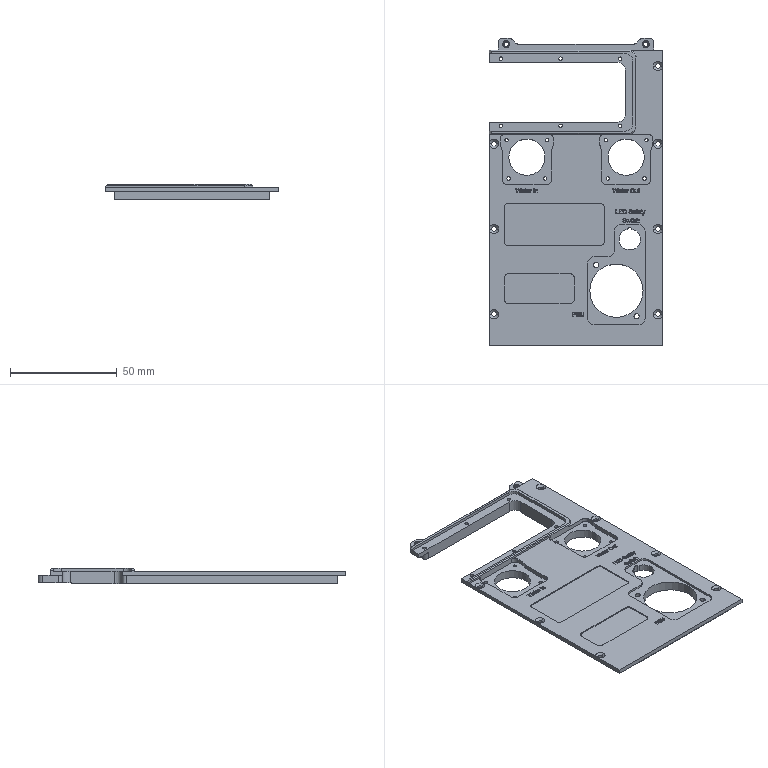NC program | NX | posted with a generic post | part box 81.5 x 144.28 x 7.5 mm
Lines 91 to 933 of 9048:
(ADAPTIVE_MILLING , TOOL : D6开粗)
N156 T01 M6
N158 G54
N160 G17 G0 G90 X-68.746 Y48.054 S6500 M3
N162 G43 Z50. H1
N164 Z-6.
N166 G94 G1 X-68.744 Y48.004 Z-6.312 F2500.
N168 X-68.741 Y47.954 Z-6.436
N170 X-68.739 Y47.904 Z-6.527
N172 X-68.736 Y47.854 Z-6.6
N174 X-68.734 Y47.804 Z-6.661
N176 X-68.731 Y47.754 Z-6.714
N178 X-68.729 Y47.704 Z-6.76
N180 X-68.727 Y47.654 Z-6.8
N182 X-68.724 Y47.604 Z-6.835
N184 X-68.722 Y47.554 Z-6.866
N186 X-68.719 Y47.504 Z-6.893
N188 X-68.717 Y47.454 Z-6.917
N190 X-68.714 Y47.404 Z-6.937
N192 X-68.712 Y47.354 Z-6.954
N194 X-68.709 Y47.305 Z-6.968
N196 X-68.707 Y47.255 Z-6.98
N198 X-68.704 Y47.205 Z-6.989
N200 X-68.702 Y47.155 Z-6.995
N202 X-68.699 Y47.105 Z-6.999
N204 X-68.697 Y47.055 Z-7.
N206 X-68.648 Y46.067
N208 G3 X-68.292 Y45.545 R0.607
N210 X-66.048 Y45.051 R6.544
N212 X-59.226 Y44.903 R95.551
N214 G1 X-55.089 Y44.901
N216 X72.351 Y44.899
N218 G2 X74.896 Y43.394 R3.392
N220 X76.098 Y40.132 R7.391
N222 X76.382 Y35.059 R37.58
N224 G1 X76.399 Y28.399
N226 X76.398 Y-40.835
N228 G2 X74.941 Y-43.359 R3.368
N230 X71.646 Y-44.596 R7.3
N232 X66.483 Y-44.883 R37.738
N234 G1 X59.103 Y-44.9
N236 X-72.29 Y-44.899
N238 G2 X-74.864 Y-43.448 R3.358
N240 X-76.09 Y-40.197 R7.25
N242 X-76.381 Y-35.079 R37.036
N244 G1 X-76.399 Y-28.149
N246 X-76.398 Y40.791
N248 G2 X-74.982 Y43.337 R3.339
N250 X-71.651 Y44.599 R7.234
N252 X-68.063 Y44.633 R12.649
N254 G3 X-59.713 Y44.31 R86.176
N256 G1 X-53.424 Y44.301
N258 X70.551 Y44.299
N260 G2 X74.189 Y42.173 R4.492
N262 X75.473 Y38.461 R9.024
N264 X75.775 Y33.209 R40.848
N266 G1 X75.799 Y25.53
N268 X75.797 Y-39.05
N270 G2 X73.654 Y-42.701 R4.49
N272 X69.98 Y-43.971 R9.023
N274 X64.233 Y-44.281 R43.718
N276 G1 X56.882 Y-44.3
N278 X-70.56 Y-44.298
N280 G2 X-72.366 Y-43.87 R5.009
N282 G1 X-72.955 Y-43.793
N284 X-73.715 Y-43.478
N286 X-74.367 Y-42.977
N288 X-74.868 Y-42.325
N290 G2 X-75.378 Y-40.504 R5.143
N292 X-75.772 Y-34.221 R45.821
N294 G1 X-75.799 Y-26.391
N296 X-75.798 Y39.061
N298 G2 X-75.25 Y41.083 R4.874
N300 G1 X-75.183 Y41.565
N302 X-74.868 Y42.325
N304 X-74.367 Y42.977
N306 X-73.715 Y43.478
N308 X-72.955 Y43.793
N310 G2 X-67.603 Y43.95 R23.279
N312 G1 X-66.688 Y43.9
N314 X66.591
N316 G3 X69.451 Y43.718 R34.087
N318 G2 X73.692 Y40.889 R5.336
N320 X74.91 Y36.767 R11.057
N322 G3 X75.195 Y35.482 R4.36
N324 G1 X75.29 Y34.499
N326 G2 X75.216 Y28.517 R176.845
N328 G1 X75.2 Y23.589
N330 X75.201 Y-30.365
N332 X75.29 Y-31.329
N334 G2 X75.184 Y-38.04 R148.514
N336 X72.364 Y-42.201 R5.303
N338 X68.371 Y-43.397 R10.985
N340 G1 X67.405 Y-43.793
N342 X66.589 Y-43.9
N344 X60.839
N346 G3 X57.254 Y-43.723 R30.565
N348 G1 X51.794 Y-43.7
N350 X33.975 Y-43.701
N352 G2 X32.839 Y-43.9 R6.236
N354 G1 X-72.141
N356 X-72.955 Y-43.793
N358 X-73.715 Y-43.478
N360 X-74.367 Y-42.977
N362 X-74.868 Y-42.325
N364 X-75.183 Y-41.565
N366 X-75.29 Y-40.749
N368 Y40.751
N370 X-75.183 Y41.565
N372 X-74.868 Y42.325
N374 X-74.367 Y42.977
N376 X-73.715 Y43.478
N378 X-72.955 Y43.793
N380 X-72.14 Y43.9
N382 X-66.65
N384 G3 X-66.063 Y44.357 R0.607
N386 G1 X-65.981 Y44.693
N388 X-65.882 Y45.024
N390 G2 X-65.333 Y45.373 R0.607
N392 G1 X-65.283 Z-6.999
N394 X-65.233 Z-6.995
N396 X-65.183 Z-6.989
N398 X-65.133 Z-6.98
N400 X-65.083 Z-6.968
N402 X-65.033 Z-6.954
N404 X-64.983 Z-6.937
N406 X-64.933 Z-6.917
N408 X-64.883 Z-6.893
N410 X-64.833 Z-6.866
N412 X-64.783 Z-6.835
N414 X-64.733 Z-6.8
N416 X-64.683 Z-6.76
N418 X-64.633 Z-6.714
N420 X-64.583 Z-6.661
N422 X-64.533 Z-6.6
N424 X-64.483 Z-6.527
N426 X-64.433 Z-6.436
N428 X-64.383 Z-6.312
N430 X-64.333 Z-6.
N432 G0 Z50.
N434 X64.727
N436 Z-6.
N438 G1 X64.777 Z-6.312
N440 X64.827 Z-6.436
N442 X64.877 Z-6.527
N444 X64.927 Z-6.6
N446 X64.977 Z-6.661
N448 X65.027 Z-6.714
N450 X65.077 Z-6.76
N452 X65.127 Z-6.8
N454 X65.177 Z-6.835
N456 X65.227 Z-6.866
N458 X65.277 Z-6.893
N460 X65.327 Z-6.917
N462 X65.377 Z-6.937
N464 X65.427 Z-6.954
N466 X65.477 Z-6.968
N468 X65.527 Z-6.98
N470 X65.577 Z-6.989
N472 X65.627 Z-6.995
N474 X65.677 Z-6.999
N476 X65.727 Z-7.
N478 G2 X66.301 Y44.962 R0.607
N480 G1 X66.542 Y44.248
N482 G3 X67.037 Y43.841 R0.607
N484 G2 X67.915 Y43.589 R2.444
N486 X70.276 Y42.804 R12.832
N488 X73.485 Y39.109 R6.8
N490 G3 X73.88 Y38.033 R13.5
N492 G2 X74.915 Y36.429 R5.884
N494 G1 X74.979 Y36.213
N496 X74.915 Y36.429
N498 G3 X73.814 Y38.112 R6.02
N500 X72.573 Y40.063 R173.318
N502 X69.102 Y42.699 R7.546
N504 G2 X68.817 Y42.977 R1.185
N506 G1 X68.165 Y43.478
N508 X67.791 Y43.633
N510 X68.165 Y43.478
N512 X68.817 Y42.977
N514 G3 X70.003 Y41.788 R6.694
N516 G2 X72.3 Y39.19 R15.9
N518 G3 X73.093 Y38.719 R15.073
N520 G1 X73.844 Y38.078
N522 G3 X72.277 Y39.181 R5.882
N524 G2 X70.58 Y40.741 R21.995
N526 X69.589 Y41.694 R16.506
N528 G1 X69.318 Y42.325
N530 X69.044 Y42.682
N532 G2 X69.555 Y41.754 R2.503
N534 G3 X71.156 Y39.578 R6.152
N536 G1 X72.311 Y39.161
N538 G3 X71.077 Y39.591 R36.922
N540 G2 X69.708 Y41.029 R3.409
N542 G1 X69.633 Y41.565
N544 G3 X69.859 Y40.484 R3.332
N546 X70.584 Y39.633 R1.822
N548 X71.293 Y39.519 R8.72
N550 G2 X70.47 Y39.659 R3.567
N552 X69.74 Y40.571 R1.303
N554 G1 X69.722 Y40.883
N556 G3 X69.767 Y40.25 R10.794
N558 X70.636 Y39.605 R0.853
N560 G2 X69.832 Y39.978 R0.96
N562 X69.74 Y40.416 R1.044
N564 G3 X69.832 Y39.978 R0.826
N566 X70.369 Y39.64 R0.728
N568 G2 X72.233 Y39.205 R5.896
N570 X73.844 Y38.078 R5.987
N572 X74.915 Y36.429 R5.987
N574 X75.29 Y34.499 R5.992
N576 G1 X75.286 Y31.283
N578 G2 X74.958 Y29.535 R5.673
N580 G3 X74.639 Y25.742 R21.469
N582 X74.6 Y18.775 R599.147
N584 G1 X74.601 Y-28.654
N586 G3 X74.992 Y-29.601 R4.451
N588 G1 X75.209 Y-30.428
N590 G3 X74.605 Y-28.761 R5.835
N592 G2 X74.307 Y-26.632 R7.842
N594 X74.239 Y-20.148 R199.676
N596 G1 X74.242 Y21.156
N598 G2 X74.404 Y27.864 R85.907
N600 X74.528 Y28.666 R3.801
N602 G3 X74.989 Y29.658 R3.993
N604 G2 X74.528 Y28.666 R3.993
N606 G3 X73.882 Y26.464 R5.45
N608 X73.65 Y20.651 R53.719
N610 G1 X73.64 Y14.365
N612 X73.642 Y-21.63
N614 G3 X73.791 Y-27.159 R61.12
N616 X73.988 Y-27.912 R1.5
N618 G2 X74.627 Y-28.801 R8.268
N620 G3 X73.898 Y-27.81 R6.471
N622 G2 X73.447 Y-25.976 R4.929
N624 X73.283 Y-20.232 R65.741
N626 G1 X73.28 Y-15.738
N628 X73.282 Y17.558
N630 G2 X73.432 Y25.243 R116.247
N632 X73.887 Y27.799 R9.722
N634 G1 X74.421 Y28.466
N636 G3 X73.542 Y27.303 R7.221
N638 X72.896 Y24.509 R8.56
N640 X72.688 Y17.82 R77.087
N642 G1 X72.68 Y11.89
N644 X72.682 Y-18.841
N646 G3 X72.825 Y-25.216 R86.495
N648 X73.151 Y-27.015 R7.72
N650 X73.934 Y-27.852 R7.987
N652 G2 X73.078 Y-26.946 R10.433
N654 X72.526 Y-24.825 R5.793
N656 G1 X72.49 Y-24.491
N658 X72.492 Y23.081
N660 G2 X73.042 Y26.737 R12.308
N662 X73.243 Y27.148 R2.48
N664 G1 X73.781 Y27.686
N666 G3 X72.831 Y26.652 R6.454
N668 X72.49 Y25.84 R2.8
N670 G1 Y22.96
N672 X72.504 Y26.094
N674 G2 X72.707 Y26.612 R1.124
N676 G1 X73.057 Y26.962
N678 G3 X72.547 Y26.372 R2.142
N680 X72.49 Y25.951 R1.722
N682 X72.79 Y25.431 R0.602
N684 G1 X72.971 Y25.326
N686 X73.443 Y25.058 Z-6.954
N688 X73.908 Y24.777 Z-6.908
N690 X73.975 Y24.713 Z-6.9
N692 G2 X74.131 Y24.31 R0.607 F15000.
N694 G1 Y-22.85
N696 G2 X73.974 Y-23.255 R0.607
N698 G1 X73.81 Y-23.383 Z-6.918 F2500.
N700 X73.63 Y-23.487 Z-6.935
N702 X72.971 Y-23.87 Z-7.
N704 X72.704 Y-24.037
N706 G3 X72.49 Y-24.491 R0.604
N708 X72.535 Y-26.276 R11.945
N710 X72.709 Y-26.614 R0.96
N712 G1 X73.186 Y-27.091
N714 G2 X72.547 Y-26.372 R3.179
N716 X72.49 Y-25.908 R1.641
N718 G3 X72.547 Y-26.372 R1.116
N720 G1 X72.709 Y-26.614
N722 G2 X74.13 Y-28.072 R49.423
N724 X75.29 Y-31.329 R5.356
N726 G1 X75.286 Y-34.546
N728 G2 X74.957 Y-36.303 R5.7
N730 X74.157 Y-38.937 R9.519
N732 X70.548 Y-41.997 R6.736
N734 G3 X69.239 Y-42.484 R25.069
N736 X68.817 Y-42.977 R2.517
N738 G1 X68.165 Y-43.478
N740 X67.999 Y-43.547
N742 X68.165 Y-43.478
N744 X68.817 Y-42.977
N746 G2 X69.794 Y-42.093 R2.317
N748 G3 X72.4 Y-40.32 R11.44
N750 X73.969 Y-37.92 R7.475
N752 X74.978 Y-36.216 R4.84
N754 G2 X73.491 Y-38.392 R4.973
N756 X70.015 Y-41.2 R19.409
N758 G3 X69.628 Y-41.576 R1.142
N760 G1 X69.318 Y-42.325
N762 X69.154 Y-42.539
N764 X69.318 Y-42.325
N766 G2 X69.732 Y-41.375 R6.637
N768 X71.329 Y-39.882 R11.928
N770 X72.09 Y-39.253 R4.923
N772 G3 X73.604 Y-38.283 R4.85
N774 G2 X71.633 Y-39.411 R4.853
N776 G3 X69.798 Y-40.736 R5.104
N778 X69.633 Y-41.565 R2.455
N780 G2 X69.782 Y-40.696 R3.509
N782 X70.945 Y-39.574 R2.827
N784 G3 X71.72 Y-39.377 R3.103
N786 G2 X70.739 Y-39.602 R3.849
N788 G3 X69.778 Y-40.339 R1.497
N790 X69.722 Y-40.885 R4.559
N792 G1 X69.744 Y-40.38
N794 G2 X70.467 Y-39.627 R1.11
N796 G1 X70.868 Y-39.575
N798 G3 X70.028 Y-39.769 R2.032
N800 X69.74 Y-40.506 R0.77
N802 G1 X69.742 Y-40.316
N804 X69.771 Y-40.128
N806 G2 X70.095 Y-39.729 R0.647
N808 X70.813 Y-39.907 R0.601
N810 G1 X70.903 Y-40.069 Z-6.984
N812 X70.964 Y-40.244 Z-6.969
N814 X71.228 Y-41.007 Z-6.9
N816 X71.456 Y-41.684 F15000.
N818 G2 X71.421 Y-42.026 R0.619
N820 G1 X71.02 Y-42.974
N822 G2 X70.083 Y-44.332 R5.029
N824 X68.796 Y-45.19 R4.206
N826 X66.517 Y-45.671 R5.796
N828 G1 X62.268 Y-45.717
N830 G2 X61.718 Y-45.387 R0.637
N832 G1 X61.039 Y-44.423 Z-7. F2500.
N834 X60.895 Y-44.215
N836 X60.742 Y-44.014
N838 G3 X60.393 Y-43.841 R0.611
N840 G2 X59.515 Y-43.589 R2.445
N842 G3 X56.197 Y-43.174 R13.991
N844 X48.014 Y-43.1 R274.433
N846 G1 X35.399 Y-43.102
N848 G3 X34.753 Y-43.219 R1.172
N850 G2 X33.791 Y-43.736 R2.658
N852 G3 X34.862 Y-43.139 R2.886
N854 G2 X36.753 Y-42.825 R6.071
N856 X44.371 Y-42.74 R173.506
N858 X55.832 Y-42.813 R388.477
N860 X58.786 Y-43.133 R14.738
N862 G1 X59.265 Y-43.478
N864 X59.639 Y-43.633
N866 G2 X58.885 Y-43.186 R1.812
N868 G3 X57.225 Y-42.526 R3.643
N870 X52.518 Y-42.174 R28.823
N872 X37.894 Y-42.197 R464.66
N874 X35.527 Y-42.494 R9.338
N876 X35.067 Y-42.977 R1.334
N878 G1 X34.817 Y-43.169
N880 G3 X35.398 Y-42.551 R2.105
N882 G2 X36.901 Y-42.034 R3.327
N884 X41.691 Y-41.792 R35.719
N886 X53.934 Y-41.865 R337.929
N888 X57.623 Y-42.333 R16.629
N890 X58.396 Y-42.695 R1.689
N892 G3 X58.72 Y-43.06 R1.419
N894 G2 X58.286 Y-42.552 R2.268
N896 G3 X56.684 Y-41.756 R3.468
N898 X52.424 Y-41.261 R20.254
N900 X39.223 Y-41.263 R237.121
N902 X36.202 Y-41.724 R10.956
N904 X35.568 Y-42.325 R0.853
N906 G1 X35.349 Y-42.611
N908 G3 X35.704 Y-42.004 R1.688
N910 G2 X36.829 Y-41.36 R2.204
N912 X40.263 Y-40.901 R14.333
N914 X53.215 Y-40.955 R179.19
N916 X56.98 Y-41.561 R14.772
N918 X57.982 Y-42.088 R2.662
N920 G1 X58.058 Y-42.199
N922 G2 X58.036 Y-42.773 R0.602
N924 G1 X57.323 Y-43.711 Z-6.9
N926 X57.175 Y-43.907 F15000.
N928 X57.018 Y-44.095
N930 G2 X56.183 Y-44.075 R0.6
N932 G1 X55.924 Y-43.799
N934 G2 X56.78 Y-42.977 R0.601
N936 G1 X57.565 Y-43.465 Z-6.978 F2500.
N938 X57.686 Y-43.502 Z-6.989
N940 X57.812 Y-43.517 Z-7.
N942 G3 X58.286 Y-42.552 R0.6
N944 G2 X57.955 Y-41.989 R2.417
N946 G3 X56.424 Y-41.034 R3.204
N948 X52.404 Y-40.371 R15.78
N950 X39.935 Y-40.346 R136.275
N952 X36.717 Y-40.93 R11.092
N954 X35.956 Y-41.409 R1.656
N956 G1 X35.893 Y-41.528
N958 G3 X36.031 Y-42.089 R0.602
N960 G1 X36.442 Y-42.428 Z-6.955
N962 X36.862 Y-42.754 Z-6.91
N964 X36.951 Y-42.825 Z-6.9
N966 X37.149 Y-42.983 F15000.
N968 X37.354 Y-43.133
N970 G3 X38.19 Y-42.854 R0.6
N972 X38.297 Y-42.427 R0.773
N974 X37.279 Y-42.056 R0.6
N976 G1 X36.634 Y-42.722 Z-6.979 F2500.
N978 X36.532 Y-42.795 Z-6.989
N980 X36.418 Y-42.847 Z-7.
N982 G2 X35.684 Y-42.045 R0.6
N984 X35.978 Y-41.329 R12.896
N986 X37.39 Y-40.502 R2.947
N988 X41.05 Y-39.965 R14.997
N990 X52.719 Y-40.055 R114.368
N992 X56.55 Y-40.796 R13.73
N994 X57.792 Y-41.58 R3.031
N996 G1 X58.023 Y-42.109
N998 G3 X57.569 Y-41.197 R3.169
N1000 X55.548 Y-40.068 R4.482
N1002 X50.943 Y-39.396 R19.77
N1004 X40.466 Y-39.435 R94.457
N1006 X37.034 Y-40.158 R11.025
N1008 X36.017 Y-40.885 R2.323
N1010 X35.883 Y-41.565 R1.943
N1012 G2 X36.02 Y-40.822 R2.538
N1014 X37.389 Y-39.806 R2.773
N1016 X40.871 Y-39.094 R12.033
N1018 X52.358 Y-39.164 R79.123
N1020 X56.191 Y-40.011 R13.29
N1022 X57.703 Y-41.123 R3.31
N1024 X57.797 Y-41.565 R2.108
N1026 G3 X57.074 Y-40.204 R1.706
N1028 X54.335 Y-38.99 R6.795
N1030 X48.879 Y-38.395 R28.557
N1032 X40.652 Y-38.555 R64.647
N1034 X37.18 Y-39.418 R10.59
N1036 X36.061 Y-40.293 R2.803
N1038 X35.99 Y-40.751 R1.027
N1040 G1 X35.955 Y-41.019
N1042 G3 X35.993 Y-40.417 R7.805
N1044 G2 X36.793 Y-39.452 R1.844
N1046 X39.81 Y-38.379 R7.689
N1048 X45.904 Y-37.998 R38.066
N1050 X52.946 Y-38.398 R47.447
N1052 X56.428 Y-39.477 R10.386
N1054 X57.645 Y-40.582 R3.196
N1056 X57.738 Y-41.115 R5.586
N1058 G3 X57.634 Y-40.39 R3.973
N1060 X56.268 Y-39.008 R3.112
N1062 X52.564 Y-37.832 R10.756
N1064 X45.076 Y-37.425 R46.446
N1066 X39.428 Y-37.921 R29.088
N1068 X36.601 Y-39.113 R6.927
N1070 X36. Y-39.871 R1.502
N1072 G1 X35.99 Y-40.493
N1074 G2 X36.026 Y-39.696 R2.952
N1076 X37.342 Y-38.414 R2.844
N1078 X41.044 Y-37.348 R10.616
N1080 X52.361 Y-37.473 R46.683
N1082 X56.231 Y-38.692 R11.214
N1084 X57.655 Y-40.082 R3.4
N1086 X57.69 Y-40.618 R2.21
N1088 G3 X57.514 Y-39.552 R1.901
N1090 X55.667 Y-37.973 R4.228
N1092 X51.46 Y-36.822 R13.486
N1094 X40.959 Y-36.812 R42.554
N1096 X37.252 Y-37.965 R10.439
N1098 X36.039 Y-39.08 R3.255
N1100 X35.99 Y-39.877 R2.523
N1102 G2 X36.025 Y-39.035 R3.31
N1104 X37.316 Y-37.698 R2.963
N1106 X40.944 Y-36.512 R10.204
N1108 X49.371 Y-36.276 R39.482
N1110 X54.58 Y-37.209 R20.359
N1112 X57.232 Y-38.825 R6.325
N1114 X57.69 Y-39.633 R1.632
N1116 G1 Y-40.083
N1118 G3 X57.597 Y-39.083 R2.531
N1120 X55.968 Y-37.407 R3.84
N1122 X51.859 Y-36.033 R11.913
N1124 X41.12 Y-35.939 R36.728
N1126 X37.297 Y-37.198 R10.694
N1128 X36.029 Y-38.407 R3.287
N1130 X35.99 Y-39.213 R3.146
N1132 G2 X36.025 Y-38.33 R3.45
N1134 X37.279 Y-36.972 R3.069
N1136 X41.031 Y-35.651 R10.228
N1138 X52.47 Y-35.826 R34.24
N1140 X56.306 Y-37.319 R10.63
N1142 X57.673 Y-38.867 R3.526
N1144 G1 X57.69 Y-39.469
N1146 G3 X57.601 Y-38.416 R2.868
N1148 X56.039 Y-36.708 R3.904
N1150 X51.897 Y-35.197 R11.655
N1152 X41.071 Y-35.102 R32.514
N1154 X37.233 Y-36.481 R10.534
N1156 X36.032 Y-37.671 R3.481
N1158 X35.99 Y-38.532 R3.193
N1160 G2 X36.026 Y-37.599 R3.628
N1162 X37.332 Y-36.173 R3.24
N1164 X41.188 Y-34.777 R10.581
N1166 X52.555 Y-35.014 R30.855
N1168 X56.389 Y-36.64 R10.425
N1170 X57.672 Y-38.167 R3.645
N1172 G1 X57.69 Y-38.821
N1174 G3 X57.607 Y-37.722 R3.227
N1176 X56.099 Y-35.992 R3.957
N1178 X52.02 Y-34.381 R11.4
N1180 X40.936 Y-34.286 R29.415
N1182 X37.153 Y-35.765 R10.287
N1184 X36.03 Y-36.926 R3.505
N1186 X35.99 Y-37.782 R3.296
N1188 G2 X36.027 Y-36.849 R3.623
N1190 X37.3 Y-35.416 R3.289
N1192 X41.222 Y-33.925 R10.618
N1194 X52.644 Y-34.206 R28.376
N1196 X56.485 Y-35.961 R10.23
N1198 X57.67 Y-37.436 R3.724
N1200 X57.69 Y-38.101 R13.552
N1202 G3 X57.632 Y-37.059 R3.744
N1204 X56.161 Y-35.266 R3.889
N1206 X52.145 Y-33.57 R11.202
N1208 X40.837 Y-33.468 R27.227
N1210 X37.047 Y-35.062 R10.069
N1212 X36.025 Y-36.177 R3.33
N1214 X35.99 Y-37.028 R3.746
N1216 G2 X36.022 Y-36.098 R4.128
N1218 X37.32 Y-34.614 R3.343
N1220 X41.25 Y-33.075 R10.746
N1222 X52.739 Y-33.401 R26.54
N1224 X56.59 Y-35.28 R10.034
N1226 X57.673 Y-36.699 R3.681
N1228 G1 X57.69 Y-37.346
N1230 G3 X57.632 Y-36.305 R3.733
N1232 X56.171 Y-34.491 R3.968
N1234 X52.119 Y-32.725 R11.278
N1236 X40.895 Y-32.614 R25.839
N1238 X37.053 Y-34.267 R10.239
N1240 X36.025 Y-35.4 R3.426
N1242 X35.99 Y-36.297 R4.029
N1244 G2 X36.023 Y-35.318 R4.301
N1246 X37.364 Y-33.785 R3.455
N1248 X41.428 Y-32.192 R11.119
N1250 X52.758 Y-32.575 R25.276
N1252 X56.521 Y-34.442 R10.254
N1254 X57.677 Y-35.952 R3.733
N1256 G1 X57.69 Y-36.581
N1258 G3 X57.631 Y-35.534 R3.738
N1260 X56.155 Y-33.687 R4.053
N1262 X51.902 Y-31.831 R11.601
N1264 X40.707 Y-31.821 R24.568
N1266 X36.942 Y-33.556 R9.908
N1268 X36.023 Y-34.617 R3.272
N1270 X35.99 Y-35.505 R4.265
N1272 G2 X36.023 Y-34.528 R4.352
N1274 X37.348 Y-32.991 R3.471
N1276 X41.524 Y-31.326 R11.236
N1278 X52.82 Y-31.76 R24.24
N1280 X56.617 Y-33.735 R10.084
N1282 X57.681 Y-35.199 R3.48
N1284 G1 X57.69 Y-35.855
N1286 G3 X57.631 Y-34.754 R4.048
N1288 X56.142 Y-32.876 R4.105
N1290 X51.962 Y-31.003 R11.625
N1292 X40.678 Y-30.99 R23.702
N1294 X36.906 Y-32.78 R9.889
N1296 X36.012 Y-33.854 R2.898
N1298 X35.99 Y-34.707 R7.384
N1300 G2 X36.022 Y-33.731 R4.493
N1302 X37.359 Y-32.171 R3.527
N1304 X41.579 Y-30.469 R11.36
N1306 X52.965 Y-30.971 R23.35
N1308 X56.657 Y-32.974 R9.945
N1310 X57.682 Y-34.421 R3.436
N1312 G1 X57.69 Y-35.068
N1314 G3 X57.634 Y-33.975 R4.203
N1316 X56.13 Y-32.059 R4.157
N1318 X51.792 Y-30.117 R11.854
N1320 X40.61 Y-30.169 R23.039
N1322 X36.909 Y-31.965 R9.9
N1324 X36.013 Y-33.043 R2.982
N1326 X35.99 Y-33.941 R6.139
N1328 G2 X36.023 Y-32.92 R4.646
N1330 X37.338 Y-31.368 R3.548
N1332 X41.553 Y-29.629 R11.33
N1334 X52.914 Y-30.119 R22.823
N1336 X56.616 Y-32.13 R10.166
N1338 X57.68 Y-33.612 R3.645
N1340 G1 X57.69 Y-34.274
N1342 G3 X57.639 Y-33.19 R4.137
N1344 X56.159 Y-31.268 R4.138
N1346 X51.819 Y-29.28 R11.814
N1348 X40.498 Y-29.362 R22.457
N1350 X36.801 Y-31.242 R9.632
N1352 X36.013 Y-32.228 R2.815
N1354 X35.99 Y-33.126 R5.965
N1356 G2 X36.023 Y-32.105 R4.646
N1358 X37.288 Y-30.584 R3.514
N1360 X41.486 Y-28.799 R11.209
N1362 X53.062 Y-29.332 R22.228
N1364 X56.751 Y-31.447 R9.814
N1366 X57.683 Y-32.827 R3.335
N1368 G1 X57.69 Y-33.465
N1370 G3 X57.631 Y-32.359 R4.163
N1372 X56.143 Y-30.436 R4.231
N1374 X51.731 Y-28.413 R11.959
N1376 X40.585 Y-28.496 R22.138
N1378 X36.855 Y-30.371 R9.886
N1380 X36.019 Y-31.392 R3.137
N1382 X35.99 Y-32.306 R3.935
N1384 G2 X36.023 Y-31.286 R4.655
N1386 X37.351 Y-29.711 R3.591
N1388 X41.651 Y-27.917 R11.52
N1390 X52.975 Y-28.464 R21.946
N1392 X56.701 Y-30.581 R10.046
N1394 X57.683 Y-32.012 R3.466
N1396 G1 X57.69 Y-32.698
N1398 G3 X57.635 Y-31.558 R4.542
N1400 X56.165 Y-29.63 R4.208
N1402 X51.838 Y-27.597 R11.845
N1404 X40.412 Y-27.707 R21.685
N1406 X36.755 Y-29.636 R9.562
N1408 X36.011 Y-30.595 R2.734
N1410 X35.99 Y-31.492 R8.887
N1412 G2 X36.02 Y-30.473 R5.101
N1414 X37.27 Y-28.944 R3.513
N1416 X41.465 Y-27.116 R11.208
N1418 X53.127 Y-27.678 R21.516
N1420 X56.753 Y-29.81 R9.869
N1422 X57.684 Y-31.2 R3.393
N1424 G1 X57.69 Y-31.882
N1426 G3 X57.64 Y-30.753 R4.787
N1428 X56.189 Y-28.823 R4.196
N1430 X51.793 Y-26.74 R11.865
N1432 X40.363 Y-26.882 R21.399
N1434 X36.785 Y-28.781 R9.607
N1436 X36.009 Y-29.777 R2.751
N1438 X35.99 Y-30.664 R13.261
N1440 G2 X36.023 Y-29.64 R4.648
N1442 X37.302 Y-28.088 R3.574
N1444 X41.509 Y-26.261 R11.344
N1446 X53.042 Y-26.808 R21.338
N1448 X56.785 Y-29.018 R9.909
N1450 X57.684 Y-30.379 R3.322
N1452 G1 X57.69 Y-31.056
N1454 G3 X57.642 Y-29.937 R4.845
N1456 X56.213 Y-28.014 R4.194
N1458 X51.903 Y-25.926 R11.733
N1460 X40.403 Y-26.028 R21.21
N1462 X36.757 Y-27.976 R9.607
N1464 X36.014 Y-28.932 R2.876
N1466 X35.99 Y-29.83 R5.557
N1468 G2 X36.023 Y-28.809 R4.64
N1470 X37.364 Y-27.209 R3.677
N1472 X41.668 Y-25.379 R11.626
N1474 X53.078 Y-25.979 R21.127
N1476 X56.793 Y-28.197 R9.896
N1478 X57.685 Y-29.565 R3.26
N1480 G1 X57.69 Y-30.24
N1482 G3 X57.642 Y-29.115 R4.629
N1484 X56.252 Y-27.214 R4.139
N1486 X51.936 Y-25.091 R11.654
N1488 X40.348 Y-25.203 R21.001
N1490 X36.758 Y-27.142 R9.605
N1492 X36.011 Y-28.111 R2.779
N1494 X35.99 Y-29.006 R9.528
N1496 G2 X36.019 Y-27.991 R5.356
N1498 X37.309 Y-26.415 R3.589
N1500 X41.596 Y-24.551 R11.47
N1502 X53.113 Y-25.151 R20.938
N1504 X56.829 Y-27.403 R9.821
N1506 X57.686 Y-28.742 R3.176
N1508 G1 X57.69 Y-29.417
N1510 G3 X57.638 Y-28.274 R4.909
N1512 X56.207 Y-26.342 R4.213
N1514 X51.816 Y-24.213 R11.853
N1516 X40.292 Y-24.38 R20.828
N1518 X36.698 Y-26.365 R9.425
N1520 X36.008 Y-27.286 R2.592
N1522 X35.99 Y-28.167 R20.937
N1524 G2 X36.023 Y-27.143 R4.583
N1526 X37.368 Y-25.533 R3.689
N1528 X41.792 Y-23.661 R11.788
N1530 X53.189 Y-24.337 R20.766
N1532 X56.788 Y-26.526 R9.852
N1534 X57.684 Y-27.895 R3.386
N1536 G1 X57.69 Y-28.572
N1538 G3 X57.643 Y-27.453 R4.575
N1540 X56.234 Y-25.528 R4.192
N1542 X51.929 Y-23.4 R11.728
N1544 X40.324 Y-23.526 R20.735
N1546 X36.709 Y-25.517 R9.512
N1548 X36.006 Y-26.463 R2.526
N1550 G1 X35.99 Y-27.328
N1552 G2 X36.023 Y-26.307 R4.654
N1554 X37.299 Y-24.748 R3.618
N1556 X41.602 Y-22.86 R11.491
N1558 X53.226 Y-23.509 R20.625
N1560 X56.827 Y-25.733 R9.763
N1562 X57.683 Y-27.053 R3.415
N1564 G1 X57.69 Y-27.74
N1566 G3 X57.64 Y-26.608 R4.845
N1568 X56.187 Y-24.65 R4.264
N1570 X51.733 Y-22.501 R11.981
N1572 X40.264 Y-22.703 R20.61
N1574 X36.679 Y-24.708 R9.408
N1576 X36.007 Y-25.62 R2.555
N1578 G1 X35.99 Y-26.494
N1580 G2 X36.023 Y-25.47 R4.588
N1582 X37.315 Y-23.897 R3.646
N1584 X41.605 Y-22.015 R11.529
N1586 X53.224 Y-22.665 R20.54
N1588 X56.843 Y-24.912 R9.727
N1590 X57.685 Y-26.232 R3.283
N1592 G1 X57.69 Y-26.907
N1594 G3 X57.636 Y-25.762 R4.737
N1596 X56.142 Y-23.774 R4.336
N1598 X51.692 Y-21.645 R12.107
N1600 X40.204 Y-21.88 R20.496
N1602 X36.654 Y-23.894 R9.307
N1604 X36.004 Y-24.795 R2.383
N1606 G1 X35.99 Y-25.652
N1608 G2 X36.023 Y-24.632 R4.657
N1610 X37.284 Y-23.08 R3.614
N1612 X41.569 Y-21.179 R11.451
N1614 X53.183 Y-21.806 R20.488
N1616 X56.805 Y-24.033 R9.855
N1618 X57.679 Y-25.359 R3.724
N1620 G1 X57.69 Y-26.076
N1622 G3 X57.641 Y-24.942 R4.663
N1624 X56.228 Y-23.006 R4.222
N1626 X51.806 Y-20.831 R11.853
N1628 X40.231 Y-21.028 R20.447
N1630 X36.663 Y-23.045 R9.372
N1632 X36.006 Y-23.947 R2.458
N1634 G1 X35.99 Y-24.814
N1636 G2 X36.023 Y-23.791 R4.618
N1638 X37.374 Y-22.17 R3.728
N1640 X41.801 Y-20.279 R11.843
N1642 X53.182 Y-20.961 R20.44
N1644 X56.821 Y-23.21 R9.851
N1646 X57.685 Y-24.559 R3.296
N1648 G1 X57.69 Y-25.234
N1650 G3 X57.638 Y-24.091 R4.847
N1652 X56.168 Y-22.115 R4.305
N1654 X51.689 Y-19.953 R12.065
N1656 X40.345 Y-20.146 R20.468
N1658 X36.75 Y-22.121 R9.671
N1660 X36.008 Y-23.1 R2.723
N1662 G1 X35.99 Y-23.978
N1664 G2 X36.02 Y-22.963 R5.173
N1666 X37.289 Y-21.395 R3.619
N1668 X41.572 Y-19.489 R11.478
N1670 X53.18 Y-20.117 R20.381
N1672 X56.842 Y-22.392 R9.801
N1674 X57.684 Y-23.707 R3.372
N1676 G1 X57.69 Y-24.387
N1678 G3 X57.642 Y-23.264 R4.586
N1680 X56.197 Y-21.297 R4.264
N1682 X51.819 Y-19.145 R11.913
N1684 X40.194 Y-19.353 R20.327
N1686 X36.68 Y-21.347 R9.384
N1688 X36.01 Y-22.253 R2.655
N1690 X35.99 Y-23.14 R12.957
N1692 G2 X36.022 Y-22.117 R4.785
N1694 X37.281 Y-20.559 R3.616
N1696 X41.573 Y-18.644 R11.467
N1698 X53.179 Y-19.273 R20.338
N1700 X56.829 Y-21.537 R9.844
N1702 X57.686 Y-22.882 R3.229
N1704 G1 X57.69 Y-23.556
N1706 G3 X57.641 Y-22.421 R4.667
N1708 X56.208 Y-20.464 R4.256
N1710 X51.725 Y-18.273 R11.973
N1712 X40.306 Y-18.471 R20.367
N1714 X36.715 Y-20.471 R9.569
N1716 X36.006 Y-21.425 R2.578
N1718 G1 X35.99 Y-22.293
N1720 G2 X36.023 Y-21.269 R4.599
N1722 X37.377 Y-19.643 R3.74
N1724 X41.805 Y-17.744 R11.863
N1726 X53.179 Y-18.428 R20.312
N1728 X56.847 Y-20.714 R9.83
N1730 X57.685 Y-22.039 R3.273
N1732 G1 X57.69 Y-22.714
N1734 G3 X57.638 Y-21.569 R4.878
N1736 X56.166 Y-19.586 R4.322
N1738 X51.608 Y-17.396 R12.15
N1740 X40.155 Y-17.679 R20.245
N1742 X36.68 Y-19.662 R9.369
N1744 X36.008 Y-20.577 R2.597
N1746 G1 X35.99 Y-21.453
N1748 G2 X36.019 Y-20.44 R5.273
N1750 X37.26 Y-18.891 R3.589
N1752 X41.537 Y-16.963 R11.391
N1754 X53.257 Y-17.614 R20.225
N1756 X56.842 Y-19.866 R9.756
N1758 X57.684 Y-21.185 R3.373
N1760 G1 X57.69 Y-21.864
N1762 G3 X57.637 Y-20.721 R4.727
N1764 X56.18 Y-18.755 R4.332
N1766 X51.724 Y-16.583 R12.041
N1768 X40.264 Y-16.797 R20.284
N1770 X36.678 Y-18.822 R9.463
N1772 X36.009 Y-19.73 R2.636
N1774 X35.99 Y-20.613 R16.343
N1776 G2 X36.021 Y-19.593 R4.915
N1778 X37.321 Y-18. R3.666
N1780 X41.624 Y-16.097 R11.596
N1782 X53.217 Y-16.754 R20.226
N1784 X56.841 Y-19.022 R9.789
N1786 X57.683 Y-20.342 R3.422
N1788 G1 X57.69 Y-21.025
N1790 G3 X57.642 Y-19.896 R4.622
N1792 X56.194 Y-17.924 R4.283
N1794 X51.8 Y-15.759 R11.947
N1796 X40.287 Y-15.945 R20.277
N1798 X36.712 Y-17.946 R9.574
N1800 X36.011 Y-18.879 R2.76
N1802 X35.99 Y-19.775 R9.381
N1804 G2 X36.018 Y-18.759 R5.499
N1806 X37.286 Y-17.184 R3.607
N1808 X41.577 Y-15.264 R11.493
N1810 X53.295 Y-15.94 R20.156
N1812 X56.85 Y-18.188 R9.719
N1814 X57.686 Y-19.516 R3.232
N1816 G1 X57.69 Y-20.19
N1818 G3 X57.638 Y-19.044 R4.581
N1820 X56.205 Y-17.089 R4.277
N1822 X51.684 Y-14.881 R12.032
N1824 X40.134 Y-15.153 R20.17
N1826 X36.667 Y-17.147 R9.33
N1828 X36.006 Y-18.053 R2.509
N1830 G1 X35.99 Y-18.923
N1832 G2 X36.023 Y-17.899 R4.589
N1834 X37.379 Y-16.269 R3.753